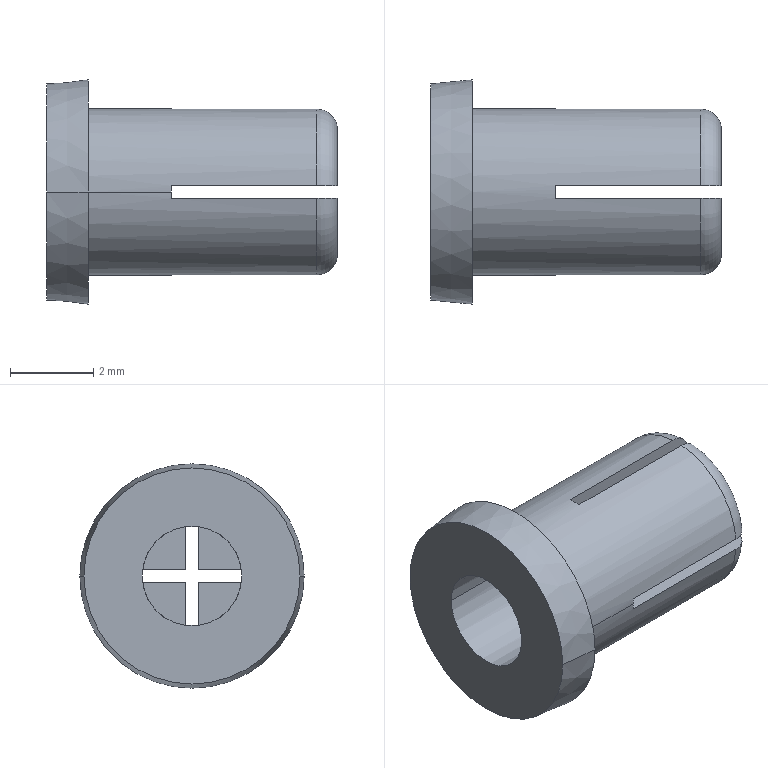Part | STEP file | SR_4060B_2 | 1 solid | 32 faces | box 7 x 5.4 x 5.4 mm | volume 66.144 mm3 | plane 22 | cylinder 4 | torus 4 | cone 2 | commonest cylinder face diameters 2.4 x2 4 x2